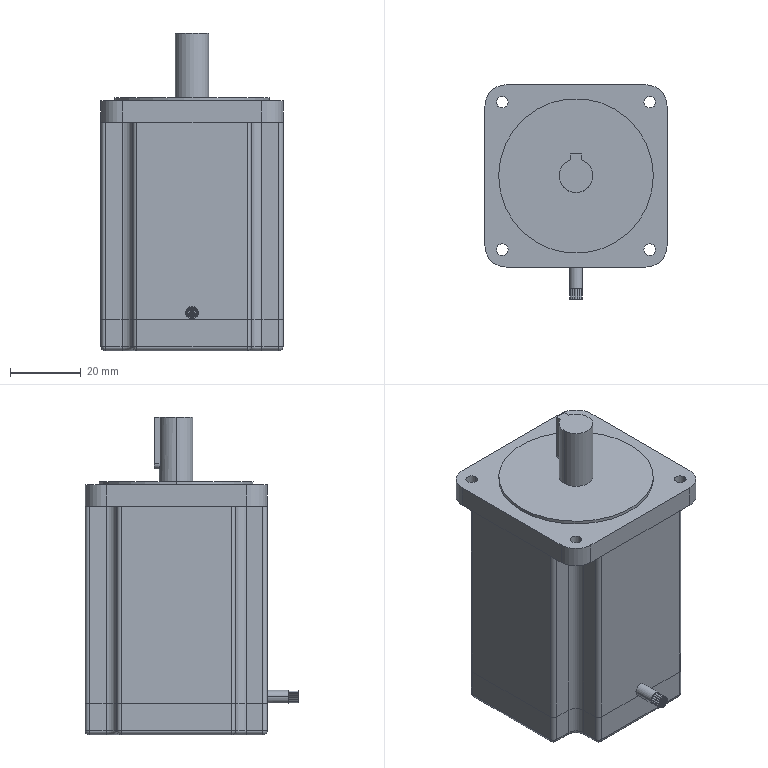Part | STEP file | MJ45 HS120 Y-axis motor | 1 solid | 169 faces | box 51.6 x 60.6 x 90 mm | volume 170208 mm3 | cylinder 96 | plane 61 | sphere 8 | torus 4 | commonest cylinder face diameters 0.6 x42 2.4 x27 3.3 x8 6 x8 12 x4 3.6 x2